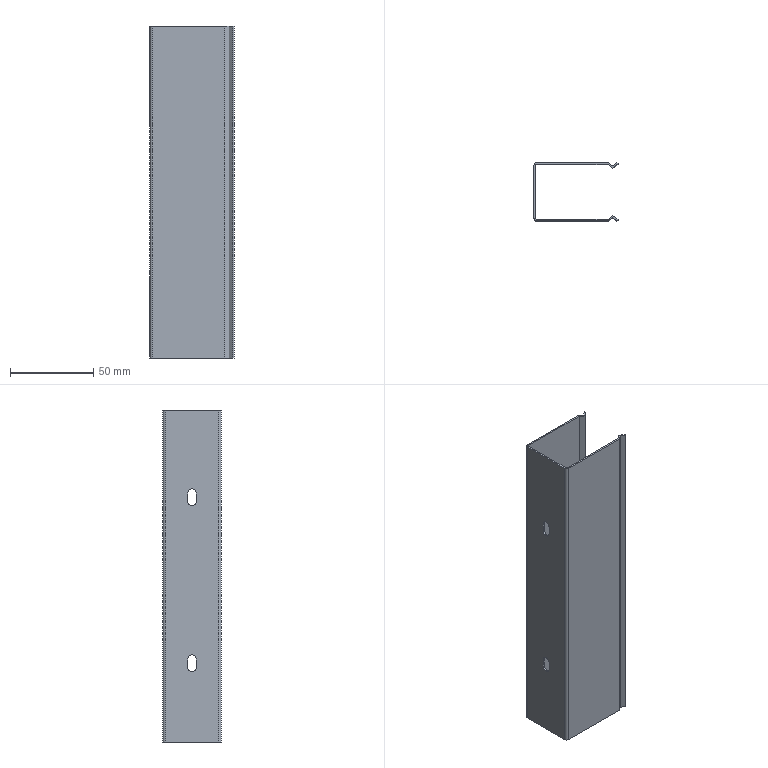Part | STEP file | 35 wire duct_200 | 1 solid | 32 faces | box 50.625 x 35 x 200 mm | volume 27080 mm3 | plane 22 | cylinder 10 | commonest cylinder face diameters 5 x6 1 x2 3 x2